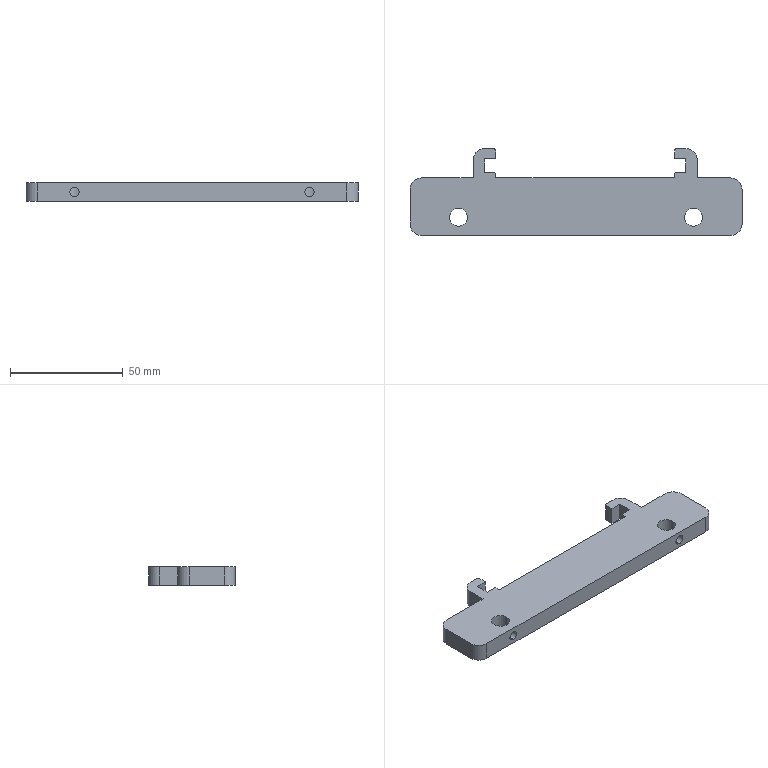Part | SolidWorks | features ICE 5, Fillet 3, Chamfer 1, Extrusion 1, HoleWzd 1, MirrorPattern 1 | 1 solid | 40 faces | box 147 x 38.4 x 8 mm | volume 30280 mm3 | plane 24 | cylinder 16 | commonest cylinder face diameters 10 x6 4.2 x4 8 x4 2 x2
STEP:
#1=CARTESIAN_POINT('',(21.5,-21.4,6.1));
#2=VERTEX_POINT('',#1);
#3=CARTESIAN_POINT('',(21.5,-21.4,1.9));
#4=VERTEX_POINT('',#3);
#5=CARTESIAN_POINT('',(21.5,-21.4,6.1));
#6=CARTESIAN_POINT('',(21.36,-21.4,6.1));
#7=CARTESIAN_POINT('',(21.219,-21.392,6.086));
#8=CARTESIAN_POINT('',(20.946,-21.364,6.03));
#9=CARTESIAN_POINT('',(20.814,-21.343,5.989));
#10=CARTESIAN_POINT('',(20.558,-21.29,5.882));
#11=CARTESIAN_POINT('',(20.438,-21.258,5.817));
#12=CARTESIAN_POINT('',(20.213,-21.189,5.665));
#13=CARTESIAN_POINT('',(20.108,-21.151,5.578));
#14=CARTESIAN_POINT('',(19.918,-21.075,5.387));
#15=CARTESIAN_POINT('',(19.833,-21.037,5.284));
#16=CARTESIAN_POINT('',(19.681,-20.964,5.058));
#17=CARTESIAN_POINT('',(19.616,-20.929,4.938));
#18=CARTESIAN_POINT('',(19.458,-20.842,4.562));
#19=CARTESIAN_POINT('',(19.4,-20.805,4.281));
#20=CARTESIAN_POINT('',(19.4,-20.804,3.864));
#21=CARTESIAN_POINT('',(19.414,-20.813,3.722));
#22=CARTESIAN_POINT('',(19.469,-20.846,3.449));
#23=CARTESIAN_POINT('',(19.509,-20.87,3.317));
#24=CARTESIAN_POINT('',(19.616,-20.929,3.063));
#25=CARTESIAN_POINT('',(19.681,-20.963,2.942));
#26=CARTESIAN_POINT('',(19.831,-21.036,2.718));
#27=CARTESIAN_POINT('',(19.918,-21.075,2.612));
#28=CARTESIAN_POINT('',(20.109,-21.152,2.421));
#29=CARTESIAN_POINT('',(20.212,-21.189,2.336));
#30=CARTESIAN_POINT('',(20.437,-21.258,2.184));
#31=CARTESIAN_POINT('',(20.559,-21.29,2.118));
#32=CARTESIAN_POINT('',(20.811,-21.342,2.011));
#33=CARTESIAN_POINT('',(20.943,-21.363,1.97));
#34=CARTESIAN_POINT('',(21.217,-21.392,1.914));
#35=CARTESIAN_POINT('',(21.359,-21.4,1.9));
#36=CARTESIAN_POINT('',(21.5,-21.4,1.9));
#37=B_SPLINE_CURVE_WITH_KNOTS('',3,(#5,#6,#7,#8,#9,#10,#11,#12,#13,#14,#15,#16,#17,#18,#19,#20,#21,#22,#23,#24,#25,#26,#27,#28,#29,#30,#31,#32,#33,#34,#35,#36),.UNSPECIFIED.,.F.,.F.,(4,2,2,2,2,2,2,2,2,2,2,2,2,2,2,4),(0.006693,0.007111,0.007528,0.007946,0.008363,0.008781,0.009198,0.01003,0.01045,0.01087,0.01129,0.0117,0.01212,0.01254,0.01296,0.01337),.UNSPECIFIED.);
#38=EDGE_CURVE('',#2,#4,#37,.T.);
#39=ORIENTED_EDGE('',*,*,#38,.F.);
#40=CARTESIAN_POINT('',(21.5,-25.4,6.1));
#41=VERTEX_POINT('',#40);
#42=CARTESIAN_POINT('',(21.5,-25.4,6.1));
#43=DIRECTION('',(0.,-1.,0.));
#44=VECTOR('',#43,1000.);
#45=LINE('',#42,#44);
#46=EDGE_CURVE('',#2,#41,#45,.T.);
#47=ORIENTED_EDGE('',*,*,#46,.T.);
#48=CARTESIAN_POINT('',(21.5,-25.4,1.9));
#49=VERTEX_POINT('',#48);
#50=CARTESIAN_POINT('',(21.5,-25.4,4.));
#51=DIRECTION('',(0.,-1.,0.));
#52=DIRECTION('',(0.,0.,-1.));
#53=AXIS2_PLACEMENT_3D('',#50,#51,#52);
#54=CIRCLE('',#53,2.1);
#55=EDGE_CURVE('',#41,#49,#54,.T.);
#56=ORIENTED_EDGE('',*,*,#55,.T.);
#57=CARTESIAN_POINT('',(21.5,-25.4,1.9));
#58=DIRECTION('',(0.,-1.,0.));
#59=VECTOR('',#58,1000.);
#60=LINE('',#57,#59);
#61=EDGE_CURVE('',#4,#49,#60,.T.);
#62=ORIENTED_EDGE('',*,*,#61,.F.);
#63=EDGE_LOOP('',(#39,#47,#56,#62));
#64=FACE_OUTER_BOUND('',#63,.T.);
#65=CARTESIAN_POINT('',(21.5,-25.4,4.));
#66=DIRECTION('',(0.,-1.,0.));
#67=DIRECTION('',(0.,0.,-1.));
#68=AXIS2_PLACEMENT_3D('',#65,#66,#67);
#69=CYLINDRICAL_SURFACE('',#68,2.1);
#70=ADVANCED_FACE('',(#64),#69,.F.);
#71=CARTESIAN_POINT('',(125.5,-21.4,6.1));
#72=VERTEX_POINT('',#71);
#73=CARTESIAN_POINT('',(125.5,-21.4,1.9));
#74=VERTEX_POINT('',#73);
#75=CARTESIAN_POINT('',(125.5,-21.4,6.1));
#76=CARTESIAN_POINT('',(125.36,-21.4,6.1));
#77=CARTESIAN_POINT('',(125.219,-21.392,6.086));
#78=CARTESIAN_POINT('',(124.946,-21.364,6.03));
#79=CARTESIAN_POINT('',(124.814,-21.343,5.989));
#80=CARTESIAN_POINT('',(124.558,-21.29,5.882));
#81=CARTESIAN_POINT('',(124.438,-21.258,5.817));
#82=CARTESIAN_POINT('',(124.213,-21.189,5.665));
#83=CARTESIAN_POINT('',(124.108,-21.151,5.578));
#84=CARTESIAN_POINT('',(123.918,-21.075,5.387));
#85=CARTESIAN_POINT('',(123.833,-21.037,5.284));
#86=CARTESIAN_POINT('',(123.681,-20.964,5.058));
#87=CARTESIAN_POINT('',(123.616,-20.929,4.938));
#88=CARTESIAN_POINT('',(123.458,-20.842,4.562));
#89=CARTESIAN_POINT('',(123.4,-20.805,4.281));
#90=CARTESIAN_POINT('',(123.4,-20.804,3.864));
#91=CARTESIAN_POINT('',(123.414,-20.813,3.722));
#92=CARTESIAN_POINT('',(123.469,-20.846,3.449));
#93=CARTESIAN_POINT('',(123.509,-20.87,3.317));
#94=CARTESIAN_POINT('',(123.616,-20.929,3.063));
#95=CARTESIAN_POINT('',(123.681,-20.963,2.942));
#96=CARTESIAN_POINT('',(123.831,-21.036,2.718));
#97=CARTESIAN_POINT('',(123.918,-21.075,2.612));
#98=CARTESIAN_POINT('',(124.109,-21.152,2.421));
#99=CARTESIAN_POINT('',(124.212,-21.189,2.336));
#100=CARTESIAN_POINT('',(124.437,-21.258,2.184));
#101=CARTESIAN_POINT('',(124.559,-21.29,2.118));
#102=CARTESIAN_POINT('',(124.811,-21.342,2.011));
#103=CARTESIAN_POINT('',(124.943,-21.363,1.97));
#104=CARTESIAN_POINT('',(125.217,-21.392,1.914));
#105=CARTESIAN_POINT('',(125.359,-21.4,1.9));
#106=CARTESIAN_POINT('',(125.5,-21.4,1.9));
#107=B_SPLINE_CURVE_WITH_KNOTS('',3,(#75,#76,#77,#78,#79,#80,#81,#82,#83,#84,#85,#86,#87,#88,#89,#90,#91,#92,#93,#94,#95,#96,#97,#98,#99,#100,#101,#102,#103,#104,#105,#106),.UNSPECIFIED.,.F.,.F.,(4,2,2,2,2,2,2,2,2,2,2,2,2,2,2,4),(0.006693,0.007111,0.007528,0.007946,0.008363,0.008781,0.009198,0.01003,0.01045,0.01087,0.01129,0.0117,0.01212,0.01254,0.01296,0.01337),.UNSPECIFIED.);
#108=EDGE_CURVE('',#72,#74,#107,.T.);
#109=ORIENTED_EDGE('',*,*,#108,.F.);
#110=CARTESIAN_POINT('',(125.5,-25.4,6.1));
#111=VERTEX_POINT('',#110);
#112=CARTESIAN_POINT('',(125.5,-25.4,6.1));
#113=DIRECTION('',(0.,-1.,0.));
#114=VECTOR('',#113,1000.);
#115=LINE('',#112,#114);
#116=EDGE_CURVE('',#72,#111,#115,.T.);
#117=ORIENTED_EDGE('',*,*,#116,.T.);
#118=CARTESIAN_POINT('',(125.5,-25.4,1.9));
#119=VERTEX_POINT('',#118);
#120=CARTESIAN_POINT('',(125.5,-25.4,4.));
#121=DIRECTION('',(0.,-1.,0.));
#122=DIRECTION('',(0.,0.,-1.));
#123=AXIS2_PLACEMENT_3D('',#120,#121,#122);
#124=CIRCLE('',#123,2.1);
#125=EDGE_CURVE('',#111,#119,#124,.T.);
#126=ORIENTED_EDGE('',*,*,#125,.T.);
#127=CARTESIAN_POINT('',(125.5,-25.4,1.9));
#128=DIRECTION('',(0.,-1.,0.));
#129=VECTOR('',#128,1000.);
#130=LINE('',#127,#129);
#131=EDGE_CURVE('',#74,#119,#130,.T.);
#132=ORIENTED_EDGE('',*,*,#131,.F.);
#133=EDGE_LOOP('',(#109,#117,#126,#132));
#134=FACE_OUTER_BOUND('',#133,.T.);
#135=CARTESIAN_POINT('',(125.5,-25.4,4.));
#136=DIRECTION('',(0.,-1.,0.));
#137=DIRECTION('',(0.,0.,-1.));
#138=AXIS2_PLACEMENT_3D('',#135,#136,#137);
#139=CYLINDRICAL_SURFACE('',#138,2.1);
#140=ADVANCED_FACE('',(#134),#139,.F.);
#141=CARTESIAN_POINT('',(21.5,-21.4,1.9));
#142=CARTESIAN_POINT('',(21.642,-21.4,1.9));
#143=CARTESIAN_POINT('',(21.78,-21.393,1.914));
#144=CARTESIAN_POINT('',(22.053,-21.364,1.969));
#145=CARTESIAN_POINT('',(22.187,-21.343,2.011));
#146=CARTESIAN_POINT('',(22.568,-21.264,2.171));
#147=CARTESIAN_POINT('',(22.797,-21.189,2.327));
#148=CARTESIAN_POINT('',(23.082,-21.075,2.612));
#149=CARTESIAN_POINT('',(23.168,-21.036,2.717));
#150=CARTESIAN_POINT('',(23.319,-20.963,2.943));
#151=CARTESIAN_POINT('',(23.384,-20.929,3.062));
#152=CARTESIAN_POINT('',(23.489,-20.871,3.313));
#153=CARTESIAN_POINT('',(23.531,-20.846,3.447));
#154=CARTESIAN_POINT('',(23.586,-20.813,3.72));
#155=CARTESIAN_POINT('',(23.6,-20.805,3.858));
#156=CARTESIAN_POINT('',(23.6,-20.804,4.138));
#157=CARTESIAN_POINT('',(23.586,-20.813,4.28));
#158=CARTESIAN_POINT('',(23.531,-20.846,4.552));
#159=CARTESIAN_POINT('',(23.49,-20.871,4.685));
#160=CARTESIAN_POINT('',(23.383,-20.929,4.939));
#161=CARTESIAN_POINT('',(23.319,-20.964,5.059));
#162=CARTESIAN_POINT('',(23.167,-21.037,5.284));
#163=CARTESIAN_POINT('',(23.08,-21.076,5.389));
#164=CARTESIAN_POINT('',(22.795,-21.19,5.675));
#165=CARTESIAN_POINT('',(22.565,-21.264,5.83));
#166=CARTESIAN_POINT('',(22.187,-21.343,5.989));
#167=CARTESIAN_POINT('',(22.053,-21.364,6.031));
#168=CARTESIAN_POINT('',(21.778,-21.393,6.086));
#169=CARTESIAN_POINT('',(21.64,-21.4,6.1));
#170=CARTESIAN_POINT('',(21.5,-21.4,6.1));
#171=B_SPLINE_CURVE_WITH_KNOTS('',3,(#141,#142,#143,#144,#145,#146,#147,#148,#149,#150,#151,#152,#153,#154,#155,#156,#157,#158,#159,#160,#161,#162,#163,#164,#165,#166,#167,#168,#169,#170),.UNSPECIFIED.,.F.,.F.,(4,2,2,2,2,2,2,2,2,2,2,2,2,2,4),(0.,0.0004183,0.0008367,0.001673,0.002092,0.00251,0.002928,0.003347,0.003765,0.004183,0.004602,0.00502,0.005857,0.006275,0.006693),.UNSPECIFIED.);
#172=EDGE_CURVE('',#4,#2,#171,.T.);
#173=ORIENTED_EDGE('',*,*,#172,.T.);
#174=ORIENTED_EDGE('',*,*,#38,.T.);
#175=EDGE_LOOP('',(#173,#174));
#176=FACE_BOUND('',#175,.T.);
#177=CARTESIAN_POINT('',(17.5,-17.4,0.));
#178=VERTEX_POINT('',#177);
#179=CARTESIAN_POINT('',(25.5,-17.4,0.));
#180=VERTEX_POINT('',#179);
#181=CARTESIAN_POINT('',(21.5,-17.4,0.));
#182=DIRECTION('',(0.,0.,1.));
#183=DIRECTION('',(1.,0.,0.));
#184=AXIS2_PLACEMENT_3D('',#181,#182,#183);
#185=CIRCLE('',#184,4.);
#186=EDGE_CURVE('',#178,#180,#185,.T.);
#187=ORIENTED_EDGE('',*,*,#186,.F.);
#188=CARTESIAN_POINT('',(17.5,-17.4,8.));
#189=VERTEX_POINT('',#188);
#190=CARTESIAN_POINT('',(17.5,-17.4,0.));
#191=DIRECTION('',(0.,0.,1.));
#192=VECTOR('',#191,1000.);
#193=LINE('',#190,#192);
#194=EDGE_CURVE('',#178,#189,#193,.T.);
#195=ORIENTED_EDGE('',*,*,#194,.T.);
#196=CARTESIAN_POINT('',(25.5,-17.4,8.));
#197=VERTEX_POINT('',#196);
#198=CARTESIAN_POINT('',(21.5,-17.4,8.));
#199=DIRECTION('',(0.,0.,1.));
#200=DIRECTION('',(1.,0.,0.));
#201=AXIS2_PLACEMENT_3D('',#198,#199,#200);
#202=CIRCLE('',#201,4.);
#203=EDGE_CURVE('',#189,#197,#202,.T.);
#204=ORIENTED_EDGE('',*,*,#203,.T.);
#205=CARTESIAN_POINT('',(25.5,-17.4,0.));
#206=DIRECTION('',(0.,0.,1.));
#207=VECTOR('',#206,1000.);
#208=LINE('',#205,#207);
#209=EDGE_CURVE('',#180,#197,#208,.T.);
#210=ORIENTED_EDGE('',*,*,#209,.F.);
#211=EDGE_LOOP('',(#187,#195,#204,#210));
#212=FACE_OUTER_BOUND('',#211,.T.);
#213=CARTESIAN_POINT('',(21.5,-17.4,0.));
#214=DIRECTION('',(0.,0.,1.));
#215=DIRECTION('',(1.,0.,0.));
#216=AXIS2_PLACEMENT_3D('',#213,#214,#215);
#217=CYLINDRICAL_SURFACE('',#216,4.);
#218=ADVANCED_FACE('',(#176,#212),#217,.F.);
#219=CARTESIAN_POINT('',(125.5,-21.4,1.9));
#220=CARTESIAN_POINT('',(125.642,-21.4,1.9));
#221=CARTESIAN_POINT('',(125.78,-21.393,1.914));
#222=CARTESIAN_POINT('',(126.053,-21.364,1.969));
#223=CARTESIAN_POINT('',(126.187,-21.343,2.011));
#224=CARTESIAN_POINT('',(126.568,-21.264,2.171));
#225=CARTESIAN_POINT('',(126.797,-21.189,2.327));
#226=CARTESIAN_POINT('',(127.082,-21.075,2.612));
#227=CARTESIAN_POINT('',(127.168,-21.036,2.717));
#228=CARTESIAN_POINT('',(127.319,-20.963,2.943));
#229=CARTESIAN_POINT('',(127.384,-20.929,3.062));
#230=CARTESIAN_POINT('',(127.489,-20.871,3.313));
#231=CARTESIAN_POINT('',(127.531,-20.846,3.447));
#232=CARTESIAN_POINT('',(127.586,-20.813,3.72));
#233=CARTESIAN_POINT('',(127.6,-20.805,3.858));
#234=CARTESIAN_POINT('',(127.6,-20.804,4.138));
#235=CARTESIAN_POINT('',(127.586,-20.813,4.28));
#236=CARTESIAN_POINT('',(127.531,-20.846,4.552));
#237=CARTESIAN_POINT('',(127.49,-20.871,4.685));
#238=CARTESIAN_POINT('',(127.383,-20.929,4.939));
#239=CARTESIAN_POINT('',(127.319,-20.964,5.059));
#240=CARTESIAN_POINT('',(127.167,-21.037,5.284));
#241=CARTESIAN_POINT('',(127.08,-21.076,5.389));
#242=CARTESIAN_POINT('',(126.795,-21.19,5.675));
#243=CARTESIAN_POINT('',(126.565,-21.264,5.83));
#244=CARTESIAN_POINT('',(126.187,-21.343,5.989));
#245=CARTESIAN_POINT('',(126.053,-21.364,6.031));
#246=CARTESIAN_POINT('',(125.778,-21.393,6.086));
#247=CARTESIAN_POINT('',(125.64,-21.4,6.1));
#248=CARTESIAN_POINT('',(125.5,-21.4,6.1));
#249=B_SPLINE_CURVE_WITH_KNOTS('',3,(#219,#220,#221,#222,#223,#224,#225,#226,#227,#228,#229,#230,#231,#232,#233,#234,#235,#236,#237,#238,#239,#240,#241,#242,#243,#244,#245,#246,#247,#248),.UNSPECIFIED.,.F.,.F.,(4,2,2,2,2,2,2,2,2,2,2,2,2,2,4),(0.,0.0004183,0.0008367,0.001673,0.002092,0.00251,0.002928,0.003347,0.003765,0.004183,0.004602,0.00502,0.005857,0.006275,0.006693),.UNSPECIFIED.);
#250=EDGE_CURVE('',#74,#72,#249,.T.);
#251=ORIENTED_EDGE('',*,*,#250,.T.);
#252=ORIENTED_EDGE('',*,*,#108,.T.);
#253=EDGE_LOOP('',(#251,#252));
#254=FACE_BOUND('',#253,.T.);
#255=CARTESIAN_POINT('',(121.5,-17.4,0.));
#256=VERTEX_POINT('',#255);
#257=CARTESIAN_POINT('',(129.5,-17.4,0.));
#258=VERTEX_POINT('',#257);
#259=CARTESIAN_POINT('',(125.5,-17.4,0.));
#260=DIRECTION('',(0.,0.,1.));
#261=DIRECTION('',(1.,0.,0.));
#262=AXIS2_PLACEMENT_3D('',#259,#260,#261);
#263=CIRCLE('',#262,4.);
#264=EDGE_CURVE('',#256,#258,#263,.T.);
#265=ORIENTED_EDGE('',*,*,#264,.F.);
#266=CARTESIAN_POINT('',(121.5,-17.4,8.));
#267=VERTEX_POINT('',#266);
#268=CARTESIAN_POINT('',(121.5,-17.4,0.));
#269=DIRECTION('',(0.,0.,1.));
#270=VECTOR('',#269,1000.);
#271=LINE('',#268,#270);
#272=EDGE_CURVE('',#256,#267,#271,.T.);
#273=ORIENTED_EDGE('',*,*,#272,.T.);
#274=CARTESIAN_POINT('',(129.5,-17.4,8.));
#275=VERTEX_POINT('',#274);
#276=CARTESIAN_POINT('',(125.5,-17.4,8.));
#277=DIRECTION('',(0.,0.,1.));
#278=DIRECTION('',(1.,0.,0.));
#279=AXIS2_PLACEMENT_3D('',#276,#277,#278);
#280=CIRCLE('',#279,4.);
#281=EDGE_CURVE('',#267,#275,#280,.T.);
#282=ORIENTED_EDGE('',*,*,#281,.T.);
#283=CARTESIAN_POINT('',(129.5,-17.4,0.));
#284=DIRECTION('',(0.,0.,1.));
#285=VECTOR('',#284,1000.);
#286=LINE('',#283,#285);
#287=EDGE_CURVE('',#258,#275,#286,.T.);
#288=ORIENTED_EDGE('',*,*,#287,.F.);
#289=EDGE_LOOP('',(#265,#273,#282,#288));
#290=FACE_OUTER_BOUND('',#289,.T.);
#291=CARTESIAN_POINT('',(125.5,-17.4,0.));
#292=DIRECTION('',(0.,0.,1.));
#293=DIRECTION('',(1.,0.,0.));
#294=AXIS2_PLACEMENT_3D('',#291,#292,#293);
#295=CYLINDRICAL_SURFACE('',#294,4.);
#296=ADVANCED_FACE('',(#254,#290),#295,.F.);
#297=CARTESIAN_POINT('',(117.2,0.,0.));
#298=VERTEX_POINT('',#297);
#299=CARTESIAN_POINT('',(117.2,0.,8.));
#300=VERTEX_POINT('',#299);
#301=CARTESIAN_POINT('',(117.2,0.,0.));
#302=DIRECTION('',(0.,0.,1.));
#303=VECTOR('',#302,1000.);
#304=LINE('',#301,#303);
#305=EDGE_CURVE('',#298,#300,#304,.T.);
#306=ORIENTED_EDGE('',*,*,#305,.F.);
#307=CARTESIAN_POINT('',(38.,0.,0.));
#308=VERTEX_POINT('',#307);
#309=CARTESIAN_POINT('',(0.,0.,0.));
#310=DIRECTION('',(-1.,0.,0.));
#311=VECTOR('',#310,1000.);
#312=LINE('',#309,#311);
#313=EDGE_CURVE('',#298,#308,#312,.T.);
#314=ORIENTED_EDGE('',*,*,#313,.T.);
#315=CARTESIAN_POINT('',(38.,0.,8.));
#316=VERTEX_POINT('',#315);
#317=CARTESIAN_POINT('',(38.,0.,0.));
#318=DIRECTION('',(0.,0.,-1.));
#319=VECTOR('',#318,1000.);
#320=LINE('',#317,#319);
#321=EDGE_CURVE('',#316,#308,#320,.T.);
#322=ORIENTED_EDGE('',*,*,#321,.F.);
#323=CARTESIAN_POINT('',(0.,0.,8.));
#324=DIRECTION('',(-1.,0.,0.));
#325=VECTOR('',#324,1000.);
#326=LINE('',#323,#325);
#327=EDGE_CURVE('',#300,#316,#326,.T.);
#328=ORIENTED_EDGE('',*,*,#327,.F.);
#329=EDGE_LOOP('',(#306,#314,#322,#328));
#330=FACE_OUTER_BOUND('',#329,.T.);
#331=CARTESIAN_POINT('',(0.,0.,8.));
#332=DIRECTION('',(0.,-1.,0.));
#333=DIRECTION('',(0.,0.,-1.));
#334=AXIS2_PLACEMENT_3D('',#331,#332,#333);
#335=PLANE('',#334);
#336=ADVANCED_FACE('',(#330),#335,.F.);
#337=CARTESIAN_POINT('',(33.,8.5,8.));
#338=VERTEX_POINT('',#337);
#339=CARTESIAN_POINT('',(33.,2.4,8.));
#340=VERTEX_POINT('',#339);
#341=CARTESIAN_POINT('',(33.,10.,8.));
#342=DIRECTION('',(0.,-1.,0.));
#343=VECTOR('',#342,1000.);
#344=LINE('',#341,#343);
#345=EDGE_CURVE('',#338,#340,#344,.T.);
#346=ORIENTED_EDGE('',*,*,#345,.T.);
#347=CARTESIAN_POINT('',(33.,2.4,0.));
#348=VERTEX_POINT('',#347);
#349=CARTESIAN_POINT('',(33.,2.4,0.));
#350=DIRECTION('',(0.,0.,1.));
#351=VECTOR('',#350,1000.);
#352=LINE('',#349,#351);
#353=EDGE_CURVE('',#348,#340,#352,.T.);
#354=ORIENTED_EDGE('',*,*,#353,.F.);
#355=CARTESIAN_POINT('',(33.,8.5,0.));
#356=VERTEX_POINT('',#355);
#357=CARTESIAN_POINT('',(33.,10.,0.));
#358=DIRECTION('',(0.,-1.,0.));
#359=VECTOR('',#358,1000.);
#360=LINE('',#357,#359);
#361=EDGE_CURVE('',#356,#348,#360,.T.);
#362=ORIENTED_EDGE('',*,*,#361,.F.);
#363=CARTESIAN_POINT('',(33.,8.5,8.));
#364=DIRECTION('',(0.,0.,-1.));
#365=VECTOR('',#364,1000.);
#366=LINE('',#363,#365);
#367=EDGE_CURVE('',#338,#356,#366,.T.);
#368=ORIENTED_EDGE('',*,*,#367,.F.);
#369=EDGE_LOOP('',(#346,#354,#362,#368));
#370=FACE_OUTER_BOUND('',#369,.T.);
#371=CARTESIAN_POINT('',(33.,10.,0.));
#372=DIRECTION('',(-1.,0.,0.));
#373=DIRECTION('',(0.,0.,1.));
#374=AXIS2_PLACEMENT_3D('',#371,#372,#373);
#375=PLANE('',#374);
#376=ADVANCED_FACE('',(#370),#375,.F.);
#377=CARTESIAN_POINT('',(28.,0.,0.));
#378=VERTEX_POINT('',#377);
#379=CARTESIAN_POINT('',(5.,0.,0.));
#380=VERTEX_POINT('',#379);
#381=CARTESIAN_POINT('',(0.,0.,0.));
#382=DIRECTION('',(-1.,0.,0.));
#383=VECTOR('',#382,1000.);
#384=LINE('',#381,#383);
#385=EDGE_CURVE('',#378,#380,#384,.T.);
#386=ORIENTED_EDGE('',*,*,#385,.T.);
#387=CARTESIAN_POINT('',(5.,0.,8.));
#388=VERTEX_POINT('',#387);
#389=CARTESIAN_POINT('',(5.,0.,8.));
#390=DIRECTION('',(0.,0.,1.));
#391=VECTOR('',#390,1000.);
#392=LINE('',#389,#391);
#393=EDGE_CURVE('',#380,#388,#392,.T.);
#394=ORIENTED_EDGE('',*,*,#393,.T.);
#395=CARTESIAN_POINT('',(28.,0.,8.));
#396=VERTEX_POINT('',#395);
#397=CARTESIAN_POINT('',(0.,0.,8.));
#398=DIRECTION('',(-1.,0.,0.));
#399=VECTOR('',#398,1000.);
#400=LINE('',#397,#399);
#401=EDGE_CURVE('',#396,#388,#400,.T.);
#402=ORIENTED_EDGE('',*,*,#401,.F.);
#403=CARTESIAN_POINT('',(28.,0.,0.));
#404=DIRECTION('',(0.,0.,1.));
#405=VECTOR('',#404,1000.);
#406=LINE('',#403,#405);
#407=EDGE_CURVE('',#378,#396,#406,.T.);
#408=ORIENTED_EDGE('',*,*,#407,.F.);
#409=EDGE_LOOP('',(#386,#394,#402,#408));
#410=FACE_OUTER_BOUND('',#409,.T.);
#411=CARTESIAN_POINT('',(0.,0.,8.));
#412=DIRECTION('',(0.,-1.,0.));
#413=DIRECTION('',(0.,0.,-1.));
#414=AXIS2_PLACEMENT_3D('',#411,#412,#413);
#415=PLANE('',#414);
#416=ADVANCED_FACE('',(#410),#415,.F.);
#417=CARTESIAN_POINT('',(142.,0.,8.));
#418=VERTEX_POINT('',#417);
#419=CARTESIAN_POINT('',(127.2,0.,8.));
#420=VERTEX_POINT('',#419);
#421=CARTESIAN_POINT('',(0.,0.,8.));
#422=DIRECTION('',(-1.,0.,0.));
#423=VECTOR('',#422,1000.);
#424=LINE('',#421,#423);
#425=EDGE_CURVE('',#418,#420,#424,.T.);
#426=ORIENTED_EDGE('',*,*,#425,.F.);
#427=CARTESIAN_POINT('',(142.,0.,0.));
#428=VERTEX_POINT('',#427);
#429=CARTESIAN_POINT('',(142.,0.,8.));
#430=DIRECTION('',(0.,0.,-1.));
#431=VECTOR('',#430,1000.);
#432=LINE('',#429,#431);
#433=EDGE_CURVE('',#418,#428,#432,.T.);
#434=ORIENTED_EDGE('',*,*,#433,.T.);
#435=CARTESIAN_POINT('',(127.2,0.,0.));
#436=VERTEX_POINT('',#435);
#437=CARTESIAN_POINT('',(0.,0.,0.));
#438=DIRECTION('',(-1.,0.,0.));
#439=VECTOR('',#438,1000.);
#440=LINE('',#437,#439);
#441=EDGE_CURVE('',#428,#436,#440,.T.);
#442=ORIENTED_EDGE('',*,*,#441,.T.);
#443=CARTESIAN_POINT('',(127.2,0.,0.));
#444=DIRECTION('',(0.,0.,-1.));
#445=VECTOR('',#444,1000.);
#446=LINE('',#443,#445);
#447=EDGE_CURVE('',#420,#436,#446,.T.);
#448=ORIENTED_EDGE('',*,*,#447,.F.);
#449=EDGE_LOOP('',(#426,#434,#442,#448));
#450=FACE_OUTER_BOUND('',#449,.T.);
#451=CARTESIAN_POINT('',(0.,0.,8.));
#452=DIRECTION('',(0.,-1.,0.));
#453=DIRECTION('',(0.,0.,-1.));
#454=AXIS2_PLACEMENT_3D('',#451,#452,#453);
#455=PLANE('',#454);
#456=ADVANCED_FACE('',(#450),#455,.F.);
#457=CARTESIAN_POINT('',(0.,-5.,0.));
#458=VERTEX_POINT('',#457);
#459=CARTESIAN_POINT('',(0.,-20.4,0.));
#460=VERTEX_POINT('',#459);
#461=CARTESIAN_POINT('',(0.,0.,0.));
#462=DIRECTION('',(0.,-1.,0.));
#463=VECTOR('',#462,1000.);
#464=LINE('',#461,#463);
#465=EDGE_CURVE('',#458,#460,#464,.T.);
#466=ORIENTED_EDGE('',*,*,#465,.T.);
#467=CARTESIAN_POINT('',(0.,-20.4,8.));
#468=VERTEX_POINT('',#467);
#469=CARTESIAN_POINT('',(0.,-20.4,8.));
#470=DIRECTION('',(0.,0.,1.));
#471=VECTOR('',#470,1000.);
#472=LINE('',#469,#471);
#473=EDGE_CURVE('',#460,#468,#472,.T.);
#474=ORIENTED_EDGE('',*,*,#473,.T.);
#475=CARTESIAN_POINT('',(0.,-5.,8.));
#476=VERTEX_POINT('',#475);
#477=CARTESIAN_POINT('',(0.,0.,8.));
#478=DIRECTION('',(0.,-1.,0.));
#479=VECTOR('',#478,1000.);
#480=LINE('',#477,#479);
#481=EDGE_CURVE('',#476,#468,#480,.T.);
#482=ORIENTED_EDGE('',*,*,#481,.F.);
#483=CARTESIAN_POINT('',(0.,-5.,8.));
#484=DIRECTION('',(0.,0.,-1.));
#485=VECTOR('',#484,1000.);
#486=LINE('',#483,#485);
#487=EDGE_CURVE('',#476,#458,#486,.T.);
#488=ORIENTED_EDGE('',*,*,#487,.T.);
#489=EDGE_LOOP('',(#466,#474,#482,#488));
#490=FACE_OUTER_BOUND('',#489,.T.);
#491=CARTESIAN_POINT('',(0.,0.,8.));
#492=DIRECTION('',(1.,0.,0.));
#493=DIRECTION('',(0.,1.,0.));
#494=AXIS2_PLACEMENT_3D('',#491,#492,#493);
#495=PLANE('',#494);
#496=ADVANCED_FACE('',(#490),#495,.F.);
#497=CARTESIAN_POINT('',(21.5,-25.4,4.));
#498=DIRECTION('',(0.,-1.,0.));
#499=DIRECTION('',(0.,0.,-1.));
#500=AXIS2_PLACEMENT_3D('',#497,#498,#499);
#501=CIRCLE('',#500,2.1);
#502=EDGE_CURVE('',#49,#41,#501,.T.);
#503=ORIENTED_EDGE('',*,*,#502,.F.);
#504=ORIENTED_EDGE('',*,*,#55,.F.);
#505=EDGE_LOOP('',(#503,#504));
#506=FACE_BOUND('',#505,.T.);
#507=CARTESIAN_POINT('',(125.5,-25.4,4.));
#508=DIRECTION('',(0.,-1.,0.));
#509=DIRECTION('',(0.,0.,-1.));
#510=AXIS2_PLACEMENT_3D('',#507,#508,#509);
#511=CIRCLE('',#510,2.1);
#512=EDGE_CURVE('',#119,#111,#511,.T.);
#513=ORIENTED_EDGE('',*,*,#512,.F.);
#514=ORIENTED_EDGE('',*,*,#125,.F.);
#515=EDGE_LOOP('',(#513,#514));
#516=FACE_BOUND('',#515,.T.);
#517=CARTESIAN_POINT('',(5.,-25.4,0.));
#518=VERTEX_POINT('',#517);
#519=CARTESIAN_POINT('',(142.,-25.4,0.));
#520=VERTEX_POINT('',#519);
#521=CARTESIAN_POINT('',(0.,-25.4,0.));
#522=DIRECTION('',(1.,0.,0.));
#523=VECTOR('',#522,1000.);
#524=LINE('',#521,#523);
#525=EDGE_CURVE('',#518,#520,#524,.T.);
#526=ORIENTED_EDGE('',*,*,#525,.T.);
#527=CARTESIAN_POINT('',(142.,-25.4,8.));
#528=VERTEX_POINT('',#527);
#529=CARTESIAN_POINT('',(142.,-25.4,8.));
#530=DIRECTION('',(0.,0.,1.));
#531=VECTOR('',#530,1000.);
#532=LINE('',#529,#531);
#533=EDGE_CURVE('',#520,#528,#532,.T.);
#534=ORIENTED_EDGE('',*,*,#533,.T.);
#535=CARTESIAN_POINT('',(5.,-25.4,8.));
#536=VERTEX_POINT('',#535);
#537=CARTESIAN_POINT('',(0.,-25.4,8.));
#538=DIRECTION('',(1.,0.,0.));
#539=VECTOR('',#538,1000.);
#540=LINE('',#537,#539);
#541=EDGE_CURVE('',#536,#528,#540,.T.);
#542=ORIENTED_EDGE('',*,*,#541,.F.);
#543=CARTESIAN_POINT('',(5.,-25.4,8.));
#544=DIRECTION('',(0.,0.,-1.));
#545=VECTOR('',#544,1000.);
#546=LINE('',#543,#545);
#547=EDGE_CURVE('',#536,#518,#546,.T.);
#548=ORIENTED_EDGE('',*,*,#547,.T.);
#549=EDGE_LOOP('',(#526,#534,#542,#548));
#550=FACE_OUTER_BOUND('',#549,.T.);
#551=CARTESIAN_POINT('',(0.,-25.4,8.));
#552=DIRECTION('',(0.,1.,0.));
#553=DIRECTION('',(0.,0.,1.));
#554=AXIS2_PLACEMENT_3D('',#551,#552,#553);
#555=PLANE('',#554);
#556=ADVANCED_FACE('',(#506,#516,#550),#555,.F.);
#557=CARTESIAN_POINT('',(147.,-20.4,8.));
#558=VERTEX_POINT('',#557);
#559=CARTESIAN_POINT('',(147.,-5.,8.));
#560=VERTEX_POINT('',#559);
#561=CARTESIAN_POINT('',(147.,0.,8.));
#562=DIRECTION('',(0.,1.,0.));
#563=VECTOR('',#562,1000.);
#564=LINE('',#561,#563);
#565=EDGE_CURVE('',#558,#560,#564,.T.);
#566=ORIENTED_EDGE('',*,*,#565,.F.);
#567=CARTESIAN_POINT('',(147.,-20.4,0.));
#568=VERTEX_POINT('',#567);
#569=CARTESIAN_POINT('',(147.,-20.4,8.));
#570=DIRECTION('',(0.,0.,-1.));
#571=VECTOR('',#570,1000.);
#572=LINE('',#569,#571);
#573=EDGE_CURVE('',#558,#568,#572,.T.);
#574=ORIENTED_EDGE('',*,*,#573,.T.);
#575=CARTESIAN_POINT('',(147.,-5.,0.));
#576=VERTEX_POINT('',#575);
#577=CARTESIAN_POINT('',(147.,0.,0.));
#578=DIRECTION('',(0.,1.,0.));
#579=VECTOR('',#578,1000.);
#580=LINE('',#577,#579);
#581=EDGE_CURVE('',#568,#576,#580,.T.);
#582=ORIENTED_EDGE('',*,*,#581,.T.);
#583=CARTESIAN_POINT('',(147.,-5.,8.));
#584=DIRECTION('',(0.,0.,1.));
#585=VECTOR('',#584,1000.);
#586=LINE('',#583,#585);
#587=EDGE_CURVE('',#576,#560,#586,.T.);
#588=ORIENTED_EDGE('',*,*,#587,.T.);
#589=EDGE_LOOP('',(#566,#574,#582,#588));
#590=FACE_OUTER_BOUND('',#589,.T.);
#591=CARTESIAN_POINT('',(147.,0.,8.));
#592=DIRECTION('',(-1.,0.,0.));
#593=DIRECTION('',(0.,0.,1.));
#594=AXIS2_PLACEMENT_3D('',#591,#592,#593);
#595=PLANE('',#594);
#596=ADVANCED_FACE('',(#590),#595,.F.);
#597=CARTESIAN_POINT('',(21.5,-17.4,8.));
#598=DIRECTION('',(0.,0.,1.));
#599=DIRECTION('',(1.,0.,0.));
#600=AXIS2_PLACEMENT_3D('',#597,#598,#599);
#601=CIRCLE('',#600,4.);
#602=EDGE_CURVE('',#197,#189,#601,.T.);
#603=ORIENTED_EDGE('',*,*,#602,.F.);
#604=ORIENTED_EDGE('',*,*,#203,.F.);
#605=EDGE_LOOP('',(#603,#604));
#606=FACE_BOUND('',#605,.T.);
#607=CARTESIAN_POINT('',(125.5,-17.4,8.));
#608=DIRECTION('',(0.,0.,1.));
#609=DIRECTION('',(1.,0.,0.));
#610=AXIS2_PLACEMENT_3D('',#607,#608,#609);
#611=CIRCLE('',#610,4.);
#612=EDGE_CURVE('',#275,#267,#611,.T.);
#613=ORIENTED_EDGE('',*,*,#612,.F.);
#614=ORIENTED_EDGE('',*,*,#281,.F.);
#615=EDGE_LOOP('',(#613,#614));
#616=FACE_BOUND('',#615,.T.);
#617=CARTESIAN_POINT('',(118.2,13.,8.));
#618=VERTEX_POINT('',#617);
#619=CARTESIAN_POINT('',(122.2,13.,8.));
#620=VERTEX_POINT('',#619);
#621=CARTESIAN_POINT('',(117.2,13.,8.));
#622=DIRECTION('',(1.,0.,0.));
#623=VECTOR('',#622,1000.);
#624=LINE('',#621,#623);
#625=EDGE_CURVE('',#618,#620,#624,.T.);
#626=ORIENTED_EDGE('',*,*,#625,.F.);
#627=CARTESIAN_POINT('',(117.2,12.,8.));
#628=VERTEX_POINT('',#627);
#629=CARTESIAN_POINT('',(118.2,12.,8.));
#630=DIRECTION('',(0.,0.,1.));
#631=DIRECTION('',(1.,0.,0.));
#632=AXIS2_PLACEMENT_3D('',#629,#630,#631);
#633=CIRCLE('',#632,1.);
#634=EDGE_CURVE('',#618,#628,#633,.T.);
#635=ORIENTED_EDGE('',*,*,#634,.T.);
#636=CARTESIAN_POINT('',(117.2,8.5,8.));
#637=VERTEX_POINT('',#636);
#638=CARTESIAN_POINT('',(117.2,10.,8.));
#639=DIRECTION('',(0.,-1.,0.));
#640=VECTOR('',#639,1000.);
#641=LINE('',#638,#640);
#642=EDGE_CURVE('',#628,#637,#641,.T.);
#643=ORIENTED_EDGE('',*,*,#642,.T.);
#644=CARTESIAN_POINT('',(122.2,8.5,8.));
#645=VERTEX_POINT('',#644);
#646=CARTESIAN_POINT('',(117.2,8.5,8.));
#647=DIRECTION('',(1.,0.,0.));
#648=VECTOR('',#647,1000.);
#649=LINE('',#646,#648);
#650=EDGE_CURVE('',#637,#645,#649,.T.);
#651=ORIENTED_EDGE('',*,*,#650,.T.);
#652=CARTESIAN_POINT('',(122.2,2.4,8.));
#653=VERTEX_POINT('',#652);
#654=CARTESIAN_POINT('',(122.2,10.,8.));
#655=DIRECTION('',(0.,-1.,0.));
#656=VECTOR('',#655,1000.);
#657=LINE('',#654,#656);
#658=EDGE_CURVE('',#645,#653,#657,.T.);
#659=ORIENTED_EDGE('',*,*,#658,.T.);
#660=CARTESIAN_POINT('',(117.7,2.4,8.));
#661=VERTEX_POINT('',#660);
#662=CARTESIAN_POINT('',(117.2,2.4,8.));
#663=DIRECTION('',(1.,0.,0.));
#664=VECTOR('',#663,1000.);
#665=LINE('',#662,#664);
#666=EDGE_CURVE('',#661,#653,#665,.T.);
#667=ORIENTED_EDGE('',*,*,#666,.F.);
#668=CARTESIAN_POINT('',(117.2,1.9,8.));
#669=VERTEX_POINT('',#668);
#670=CARTESIAN_POINT('',(57.65,-57.65,8.));
#671=DIRECTION('',(-0.7071,-0.7071,0.));
#672=VECTOR('',#671,1000.);
#673=LINE('',#670,#672);
#674=EDGE_CURVE('',#661,#669,#673,.T.);
#675=ORIENTED_EDGE('',*,*,#674,.T.);
#676=CARTESIAN_POINT('',(117.2,2.4,8.));
#677=DIRECTION('',(0.,-1.,0.));
#678=VECTOR('',#677,1000.);
#679=LINE('',#676,#678);
#680=EDGE_CURVE('',#669,#300,#679,.T.);
#681=ORIENTED_EDGE('',*,*,#680,.T.);
#682=ORIENTED_EDGE('',*,*,#327,.T.);
#683=CARTESIAN_POINT('',(38.,1.9,8.));
#684=VERTEX_POINT('',#683);
#685=CARTESIAN_POINT('',(38.,2.4,8.));
#686=DIRECTION('',(0.,-1.,0.));
#687=VECTOR('',#686,1000.);
#688=LINE('',#685,#687);
#689=EDGE_CURVE('',#684,#316,#688,.T.);
#690=ORIENTED_EDGE('',*,*,#689,.F.);
#691=CARTESIAN_POINT('',(37.5,2.4,8.));
#692=VERTEX_POINT('',#691);
#693=CARTESIAN_POINT('',(19.95,19.95,8.));
#694=DIRECTION('',(-0.7071,0.7071,0.));
#695=VECTOR('',#694,1000.);
#696=LINE('',#693,#695);
#697=EDGE_CURVE('',#684,#692,#696,.T.);
#698=ORIENTED_EDGE('',*,*,#697,.T.);
#699=CARTESIAN_POINT('',(33.,2.4,8.));
#700=DIRECTION('',(1.,0.,0.));
#701=VECTOR('',#700,1000.);
#702=LINE('',#699,#701);
#703=EDGE_CURVE('',#340,#692,#702,.T.);
#704=ORIENTED_EDGE('',*,*,#703,.F.);
#705=ORIENTED_EDGE('',*,*,#345,.F.);
#706=CARTESIAN_POINT('',(38.,8.5,8.));
#707=VERTEX_POINT('',#706);
#708=CARTESIAN_POINT('',(38.,8.5,8.));
#709=DIRECTION('',(-1.,0.,0.));
#710=VECTOR('',#709,1000.);
#711=LINE('',#708,#710);
#712=EDGE_CURVE('',#707,#338,#711,.T.);
#713=ORIENTED_EDGE('',*,*,#712,.F.);
#714=CARTESIAN_POINT('',(38.,12.,8.));
#715=VERTEX_POINT('',#714);
#716=CARTESIAN_POINT('',(38.,10.,8.));
#717=DIRECTION('',(0.,-1.,0.));
#718=VECTOR('',#717,1000.);
#719=LINE('',#716,#718);
#720=EDGE_CURVE('',#715,#707,#719,.T.);
#721=ORIENTED_EDGE('',*,*,#720,.F.);
#722=CARTESIAN_POINT('',(37.,13.,8.));
#723=VERTEX_POINT('',#722);
#724=CARTESIAN_POINT('',(37.,12.,8.));
#725=DIRECTION('',(0.,0.,1.));
#726=DIRECTION('',(1.,0.,0.));
#727=AXIS2_PLACEMENT_3D('',#724,#725,#726);
#728=CIRCLE('',#727,1.);
#729=EDGE_CURVE('',#715,#723,#728,.T.);
#730=ORIENTED_EDGE('',*,*,#729,.T.);
#731=CARTESIAN_POINT('',(33.,13.,8.));
#732=VERTEX_POINT('',#731);
#733=CARTESIAN_POINT('',(28.,13.,8.));
#734=DIRECTION('',(1.,0.,0.));
#735=VECTOR('',#734,1000.);
#736=LINE('',#733,#735);
#737=EDGE_CURVE('',#732,#723,#736,.T.);
#738=ORIENTED_EDGE('',*,*,#737,.F.);
#739=CARTESIAN_POINT('',(28.,8.,8.));
#740=VERTEX_POINT('',#739);
#741=CARTESIAN_POINT('',(33.,8.,8.));
#742=DIRECTION('',(0.,0.,1.));
#743=DIRECTION('',(1.,0.,0.));
#744=AXIS2_PLACEMENT_3D('',#741,#742,#743);
#745=CIRCLE('',#744,5.);
#746=EDGE_CURVE('',#732,#740,#745,.T.);
#747=ORIENTED_EDGE('',*,*,#746,.T.);
#748=CARTESIAN_POINT('',(28.,10.,8.));
#749=DIRECTION('',(0.,-1.,0.));
#750=VECTOR('',#749,1000.);
#751=LINE('',#748,#750);
#752=EDGE_CURVE('',#740,#396,#751,.T.);
#753=ORIENTED_EDGE('',*,*,#752,.T.);
#754=ORIENTED_EDGE('',*,*,#401,.T.);
#755=CARTESIAN_POINT('',(5.,-5.,8.));
#756=DIRECTION('',(0.,0.,1.));
#757=DIRECTION('',(1.,0.,0.));
#758=AXIS2_PLACEMENT_3D('',#755,#756,#757);
#759=CIRCLE('',#758,5.);
#760=EDGE_CURVE('',#388,#476,#759,.T.);
#761=ORIENTED_EDGE('',*,*,#760,.T.);
#762=ORIENTED_EDGE('',*,*,#481,.T.);
#763=CARTESIAN_POINT('',(5.,-20.4,8.));
#764=DIRECTION('',(0.,0.,1.));
#765=DIRECTION('',(1.,0.,0.));
#766=AXIS2_PLACEMENT_3D('',#763,#764,#765);
#767=CIRCLE('',#766,5.);
#768=EDGE_CURVE('',#468,#536,#767,.T.);
#769=ORIENTED_EDGE('',*,*,#768,.T.);
#770=ORIENTED_EDGE('',*,*,#541,.T.);
#771=CARTESIAN_POINT('',(142.,-20.4,8.));
#772=DIRECTION('',(0.,0.,1.));
#773=DIRECTION('',(1.,0.,0.));
#774=AXIS2_PLACEMENT_3D('',#771,#772,#773);
#775=CIRCLE('',#774,5.);
#776=EDGE_CURVE('',#528,#558,#775,.T.);
#777=ORIENTED_EDGE('',*,*,#776,.T.);
#778=ORIENTED_EDGE('',*,*,#565,.T.);
#779=CARTESIAN_POINT('',(142.,-5.,8.));
#780=DIRECTION('',(0.,0.,1.));
#781=DIRECTION('',(1.,0.,0.));
#782=AXIS2_PLACEMENT_3D('',#779,#780,#781);
#783=CIRCLE('',#782,5.);
#784=EDGE_CURVE('',#560,#418,#783,.T.);
#785=ORIENTED_EDGE('',*,*,#784,.T.);
#786=ORIENTED_EDGE('',*,*,#425,.T.);
#787=CARTESIAN_POINT('',(127.2,8.,8.));
#788=VERTEX_POINT('',#787);
#789=CARTESIAN_POINT('',(127.2,10.,8.));
#790=DIRECTION('',(0.,-1.,0.));
#791=VECTOR('',#790,1000.);
#792=LINE('',#789,#791);
#793=EDGE_CURVE('',#788,#420,#792,.T.);
#794=ORIENTED_EDGE('',*,*,#793,.F.);
#795=CARTESIAN_POINT('',(122.2,8.,8.));
#796=DIRECTION('',(0.,0.,1.));
#797=DIRECTION('',(1.,0.,0.));
#798=AXIS2_PLACEMENT_3D('',#795,#796,#797);
#799=CIRCLE('',#798,5.);
#800=EDGE_CURVE('',#788,#620,#799,.T.);
#801=ORIENTED_EDGE('',*,*,#800,.T.);
#802=EDGE_LOOP('',(#626,#635,#643,#651,#659,#667,#675,#681,#682,#690,#698,#704,#705,#713,#721,#730,#738,#747,#753,#754,#761,#762,#769,#770,#777,#778,#785,#786,#794,#801));
#803=FACE_OUTER_BOUND('',#802,.T.);
#804=CARTESIAN_POINT('',(0.,0.,8.));
#805=DIRECTION('',(0.,0.,1.));
#806=DIRECTION('',(1.,0.,0.));
#807=AXIS2_PLACEMENT_3D('',#804,#805,#806);
#808=PLANE('',#807);
#809=ADVANCED_FACE('',(#606,#616,#803),#808,.T.);
#810=CARTESIAN_POINT('',(21.5,-17.4,0.));
#811=DIRECTION('',(0.,0.,1.));
#812=DIRECTION('',(1.,0.,0.));
#813=AXIS2_PLACEMENT_3D('',#810,#811,#812);
#814=CIRCLE('',#813,4.);
#815=EDGE_CURVE('',#180,#178,#814,.T.);
#816=ORIENTED_EDGE('',*,*,#815,.T.);
#817=ORIENTED_EDGE('',*,*,#186,.T.);
#818=EDGE_LOOP('',(#816,#817));
#819=FACE_BOUND('',#818,.T.);
#820=CARTESIAN_POINT('',(125.5,-17.4,0.));
#821=DIRECTION('',(0.,0.,1.));
#822=DIRECTION('',(1.,0.,0.));
#823=AXIS2_PLACEMENT_3D('',#820,#821,#822);
#824=CIRCLE('',#823,4.);
#825=EDGE_CURVE('',#258,#256,#824,.T.);
#826=ORIENTED_EDGE('',*,*,#825,.T.);
#827=ORIENTED_EDGE('',*,*,#264,.T.);
#828=EDGE_LOOP('',(#826,#827));
#829=FACE_BOUND('',#828,.T.);
#830=CARTESIAN_POINT('',(117.2,8.5,0.));
#831=VERTEX_POINT('',#830);
#832=CARTESIAN_POINT('',(117.2,12.,0.));
#833=VERTEX_POINT('',#832);
#834=CARTESIAN_POINT('',(117.2,10.,0.));
#835=DIRECTION('',(0.,1.,0.));
#836=VECTOR('',#835,1000.);
#837=LINE('',#834,#836);
#838=EDGE_CURVE('',#831,#833,#837,.T.);
#839=ORIENTED_EDGE('',*,*,#838,.T.);
#840=CARTESIAN_POINT('',(118.2,13.,0.));
#841=VERTEX_POINT('',#840);
#842=CARTESIAN_POINT('',(118.2,12.,0.));
#843=DIRECTION('',(0.,0.,-1.));
#844=DIRECTION('',(1.,0.,0.));
#845=AXIS2_PLACEMENT_3D('',#842,#843,#844);
#846=CIRCLE('',#845,1.);
#847=EDGE_CURVE('',#833,#841,#846,.T.);
#848=ORIENTED_EDGE('',*,*,#847,.T.);
#849=CARTESIAN_POINT('',(122.2,13.,0.));
#850=VERTEX_POINT('',#849);
#851=CARTESIAN_POINT('',(127.2,13.,0.));
#852=DIRECTION('',(-1.,0.,0.));
#853=VECTOR('',#852,1000.);
#854=LINE('',#851,#853);
#855=EDGE_CURVE('',#850,#841,#854,.T.);
#856=ORIENTED_EDGE('',*,*,#855,.F.);
#857=CARTESIAN_POINT('',(127.2,8.,0.));
#858=VERTEX_POINT('',#857);
#859=CARTESIAN_POINT('',(122.2,8.,0.));
#860=DIRECTION('',(0.,0.,-1.));
#861=DIRECTION('',(1.,0.,0.));
#862=AXIS2_PLACEMENT_3D('',#859,#860,#861);
#863=CIRCLE('',#862,5.);
#864=EDGE_CURVE('',#850,#858,#863,.T.);
#865=ORIENTED_EDGE('',*,*,#864,.T.);
#866=CARTESIAN_POINT('',(127.2,10.,0.));
#867=DIRECTION('',(0.,-1.,0.));
#868=VECTOR('',#867,1000.);
#869=LINE('',#866,#868);
#870=EDGE_CURVE('',#858,#436,#869,.T.);
#871=ORIENTED_EDGE('',*,*,#870,.T.);
#872=ORIENTED_EDGE('',*,*,#441,.F.);
#873=CARTESIAN_POINT('',(142.,-5.,0.));
#874=DIRECTION('',(0.,0.,-1.));
#875=DIRECTION('',(1.,0.,0.));
#876=AXIS2_PLACEMENT_3D('',#873,#874,#875);
#877=CIRCLE('',#876,5.);
#878=EDGE_CURVE('',#428,#576,#877,.T.);
#879=ORIENTED_EDGE('',*,*,#878,.T.);
#880=ORIENTED_EDGE('',*,*,#581,.F.);
#881=CARTESIAN_POINT('',(142.,-20.4,0.));
#882=DIRECTION('',(0.,0.,-1.));
#883=DIRECTION('',(1.,0.,0.));
#884=AXIS2_PLACEMENT_3D('',#881,#882,#883);
#885=CIRCLE('',#884,5.);
#886=EDGE_CURVE('',#568,#520,#885,.T.);
#887=ORIENTED_EDGE('',*,*,#886,.T.);
#888=ORIENTED_EDGE('',*,*,#525,.F.);
#889=CARTESIAN_POINT('',(5.,-20.4,0.));
#890=DIRECTION('',(0.,0.,-1.));
#891=DIRECTION('',(1.,0.,0.));
#892=AXIS2_PLACEMENT_3D('',#889,#890,#891);
#893=CIRCLE('',#892,5.);
#894=EDGE_CURVE('',#518,#460,#893,.T.);
#895=ORIENTED_EDGE('',*,*,#894,.T.);
#896=ORIENTED_EDGE('',*,*,#465,.F.);
#897=CARTESIAN_POINT('',(5.,-5.,0.));
#898=DIRECTION('',(0.,0.,-1.));
#899=DIRECTION('',(1.,0.,0.));
#900=AXIS2_PLACEMENT_3D('',#897,#898,#899);
#901=CIRCLE('',#900,5.);
#902=EDGE_CURVE('',#458,#380,#901,.T.);
#903=ORIENTED_EDGE('',*,*,#902,.T.);
#904=ORIENTED_EDGE('',*,*,#385,.F.);
#905=CARTESIAN_POINT('',(28.,8.,0.));
#906=VERTEX_POINT('',#905);
#907=CARTESIAN_POINT('',(28.,10.,0.));
#908=DIRECTION('',(0.,-1.,0.));
#909=VECTOR('',#908,1000.);
#910=LINE('',#907,#909);
#911=EDGE_CURVE('',#906,#378,#910,.T.);
#912=ORIENTED_EDGE('',*,*,#911,.F.);
#913=CARTESIAN_POINT('',(33.,13.,0.));
#914=VERTEX_POINT('',#913);
#915=CARTESIAN_POINT('',(33.,8.,0.));
#916=DIRECTION('',(0.,0.,-1.));
#917=DIRECTION('',(1.,0.,0.));
#918=AXIS2_PLACEMENT_3D('',#915,#916,#917);
#919=CIRCLE('',#918,5.);
#920=EDGE_CURVE('',#906,#914,#919,.T.);
#921=ORIENTED_EDGE('',*,*,#920,.T.);
#922=CARTESIAN_POINT('',(37.,13.,0.));
#923=VERTEX_POINT('',#922);
#924=CARTESIAN_POINT('',(38.,13.,0.));
#925=DIRECTION('',(-1.,0.,0.));
#926=VECTOR('',#925,1000.);
#927=LINE('',#924,#926);
#928=EDGE_CURVE('',#923,#914,#927,.T.);
#929=ORIENTED_EDGE('',*,*,#928,.F.);
#930=CARTESIAN_POINT('',(38.,12.,0.));
#931=VERTEX_POINT('',#930);
#932=CARTESIAN_POINT('',(37.,12.,0.));
#933=DIRECTION('',(0.,0.,-1.));
#934=DIRECTION('',(1.,0.,0.));
#935=AXIS2_PLACEMENT_3D('',#932,#933,#934);
#936=CIRCLE('',#935,1.);
#937=EDGE_CURVE('',#923,#931,#936,.T.);
#938=ORIENTED_EDGE('',*,*,#937,.T.);
#939=CARTESIAN_POINT('',(38.,8.5,0.));
#940=VERTEX_POINT('',#939);
#941=CARTESIAN_POINT('',(38.,10.,0.));
#942=DIRECTION('',(0.,1.,0.));
#943=VECTOR('',#942,1000.);
#944=LINE('',#941,#943);
#945=EDGE_CURVE('',#940,#931,#944,.T.);
#946=ORIENTED_EDGE('',*,*,#945,.F.);
#947=CARTESIAN_POINT('',(38.,8.5,0.));
#948=DIRECTION('',(-1.,0.,0.));
#949=VECTOR('',#948,1000.);
#950=LINE('',#947,#949);
#951=EDGE_CURVE('',#940,#356,#950,.T.);
#952=ORIENTED_EDGE('',*,*,#951,.T.);
#953=ORIENTED_EDGE('',*,*,#361,.T.);
#954=CARTESIAN_POINT('',(37.5,2.4,0.));
#955=VERTEX_POINT('',#954);
#956=CARTESIAN_POINT('',(33.,2.4,0.));
#957=DIRECTION('',(-1.,0.,0.));
#958=VECTOR('',#957,1000.);
#959=LINE('',#956,#958);
#960=EDGE_CURVE('',#955,#348,#959,.T.);
#961=ORIENTED_EDGE('',*,*,#960,.F.);
#962=CARTESIAN_POINT('',(38.,1.9,0.));
#963=VERTEX_POINT('',#962);
#964=CARTESIAN_POINT('',(37.5,2.4,0.));
#965=DIRECTION('',(0.7071,-0.7071,0.));
#966=VECTOR('',#965,1000.);
#967=LINE('',#964,#966);
#968=EDGE_CURVE('',#955,#963,#967,.T.);
#969=ORIENTED_EDGE('',*,*,#968,.T.);
#970=CARTESIAN_POINT('',(38.,2.4,0.));
#971=DIRECTION('',(0.,-1.,0.));
#972=VECTOR('',#971,1000.);
#973=LINE('',#970,#972);
#974=EDGE_CURVE('',#963,#308,#973,.T.);
#975=ORIENTED_EDGE('',*,*,#974,.T.);
#976=ORIENTED_EDGE('',*,*,#313,.F.);
#977=CARTESIAN_POINT('',(117.2,1.9,0.));
#978=VERTEX_POINT('',#977);
#979=CARTESIAN_POINT('',(117.2,2.4,0.));
#980=DIRECTION('',(0.,-1.,0.));
#981=VECTOR('',#980,1000.);
#982=LINE('',#979,#981);
#983=EDGE_CURVE('',#978,#298,#982,.T.);
#984=ORIENTED_EDGE('',*,*,#983,.F.);
#985=CARTESIAN_POINT('',(117.7,2.4,0.));
#986=VERTEX_POINT('',#985);
#987=CARTESIAN_POINT('',(117.7,2.4,0.));
#988=DIRECTION('',(0.7071,0.7071,0.));
#989=VECTOR('',#988,1000.);
#990=LINE('',#987,#989);
#991=EDGE_CURVE('',#978,#986,#990,.T.);
#992=ORIENTED_EDGE('',*,*,#991,.T.);
#993=CARTESIAN_POINT('',(122.2,2.4,0.));
#994=VERTEX_POINT('',#993);
#995=CARTESIAN_POINT('',(117.2,2.4,0.));
#996=DIRECTION('',(-1.,0.,0.));
#997=VECTOR('',#996,1000.);
#998=LINE('',#995,#997);
#999=EDGE_CURVE('',#994,#986,#998,.T.);
#1000=ORIENTED_EDGE('',*,*,#999,.F.);
#1001=CARTESIAN_POINT('',(122.2,8.5,0.));
#1002=VERTEX_POINT('',#1001);
#1003=CARTESIAN_POINT('',(122.2,10.,0.));
#1004=DIRECTION('',(0.,-1.,0.));
#1005=VECTOR('',#1004,1000.);
#1006=LINE('',#1003,#1005);
#1007=EDGE_CURVE('',#1002,#994,#1006,.T.);
#1008=ORIENTED_EDGE('',*,*,#1007,.F.);
#1009=CARTESIAN_POINT('',(117.2,8.5,0.));
#1010=DIRECTION('',(1.,0.,0.));
#1011=VECTOR('',#1010,1000.);
#1012=LINE('',#1009,#1011);
#1013=EDGE_CURVE('',#831,#1002,#1012,.T.);
#1014=ORIENTED_EDGE('',*,*,#1013,.F.);
#1015=EDGE_LOOP('',(#839,#848,#856,#865,#871,#872,#879,#880,#887,#888,#895,#896,#903,#904,#912,#921,#929,#938,#946,#952,#953,#961,#969,#975,#976,#984,#992,#1000,#1008,#1014));
#1016=FACE_OUTER_BOUND('',#1015,.T.);
#1017=CARTESIAN_POINT('',(0.,0.,0.));
#1018=DIRECTION('',(0.,0.,1.));
#1019=DIRECTION('',(1.,0.,0.));
#1020=AXIS2_PLACEMENT_3D('',#1017,#1018,#1019);
#1021=PLANE('',#1020);
#1022=ADVANCED_FACE('',(#819,#829,#1016),#1021,.F.);
#1023=ORIENTED_EDGE('',*,*,#1007,.T.);
#1024=CARTESIAN_POINT('',(122.2,2.4,0.));
#1025=DIRECTION('',(0.,0.,-1.));
#1026=VECTOR('',#1025,1000.);
#1027=LINE('',#1024,#1026);
#1028=EDGE_CURVE('',#653,#994,#1027,.T.);
#1029=ORIENTED_EDGE('',*,*,#1028,.F.);
#1030=ORIENTED_EDGE('',*,*,#658,.F.);
#1031=CARTESIAN_POINT('',(122.2,8.5,8.));
#1032=DIRECTION('',(0.,0.,-1.));
#1033=VECTOR('',#1032,1000.);
#1034=LINE('',#1031,#1033);
#1035=EDGE_CURVE('',#645,#1002,#1034,.T.);
#1036=ORIENTED_EDGE('',*,*,#1035,.T.);
#1037=EDGE_LOOP('',(#1023,#1029,#1030,#1036));
#1038=FACE_OUTER_BOUND('',#1037,.T.);
#1039=CARTESIAN_POINT('',(122.2,10.,0.));
#1040=DIRECTION('',(1.,0.,0.));
#1041=DIRECTION('',(0.,0.,-1.));
#1042=AXIS2_PLACEMENT_3D('',#1039,#1040,#1041);
#1043=PLANE('',#1042);
#1044=ADVANCED_FACE('',(#1038),#1043,.F.);
#1045=ORIENTED_EDGE('',*,*,#870,.F.);
#1046=CARTESIAN_POINT('',(127.2,8.,8.));
#1047=DIRECTION('',(0.,0.,1.));
#1048=VECTOR('',#1047,1000.);
#1049=LINE('',#1046,#1048);
#1050=EDGE_CURVE('',#858,#788,#1049,.T.);
#1051=ORIENTED_EDGE('',*,*,#1050,.T.);
#1052=ORIENTED_EDGE('',*,*,#793,.T.);
#1053=ORIENTED_EDGE('',*,*,#447,.T.);
#1054=EDGE_LOOP('',(#1045,#1051,#1052,#1053));
#1055=FACE_OUTER_BOUND('',#1054,.T.);
#1056=CARTESIAN_POINT('',(127.2,10.,0.));
#1057=DIRECTION('',(-1.,0.,0.));
#1058=DIRECTION('',(0.,0.,1.));
#1059=AXIS2_PLACEMENT_3D('',#1056,#1057,#1058);
#1060=PLANE('',#1059);
#1061=ADVANCED_FACE('',(#1055),#1060,.F.);
#1062=ORIENTED_EDGE('',*,*,#752,.F.);
#1063=CARTESIAN_POINT('',(28.,8.,0.));
#1064=DIRECTION('',(0.,0.,-1.));
#1065=VECTOR('',#1064,1000.);
#1066=LINE('',#1063,#1065);
#1067=EDGE_CURVE('',#740,#906,#1066,.T.);
#1068=ORIENTED_EDGE('',*,*,#1067,.T.);
#1069=ORIENTED_EDGE('',*,*,#911,.T.);
#1070=ORIENTED_EDGE('',*,*,#407,.T.);
#1071=EDGE_LOOP('',(#1062,#1068,#1069,#1070));
#1072=FACE_OUTER_BOUND('',#1071,.T.);
#1073=CARTESIAN_POINT('',(28.,10.,0.));
#1074=DIRECTION('',(1.,0.,0.));
#1075=DIRECTION('',(0.,0.,-1.));
#1076=AXIS2_PLACEMENT_3D('',#1073,#1074,#1075);
#1077=PLANE('',#1076);
#1078=ADVANCED_FACE('',(#1072),#1077,.F.);
#1079=ORIENTED_EDGE('',*,*,#367,.T.);
#1080=ORIENTED_EDGE('',*,*,#951,.F.);
#1081=CARTESIAN_POINT('',(38.,8.5,8.));
#1082=DIRECTION('',(0.,0.,-1.));
#1083=VECTOR('',#1082,1000.);
#1084=LINE('',#1081,#1083);
#1085=EDGE_CURVE('',#707,#940,#1084,.T.);
#1086=ORIENTED_EDGE('',*,*,#1085,.F.);
#1087=ORIENTED_EDGE('',*,*,#712,.T.);
#1088=EDGE_LOOP('',(#1079,#1080,#1086,#1087));
#1089=FACE_OUTER_BOUND('',#1088,.T.);
#1090=CARTESIAN_POINT('',(38.,8.5,8.));
#1091=DIRECTION('',(0.,1.,0.));
#1092=DIRECTION('',(0.,0.,1.));
#1093=AXIS2_PLACEMENT_3D('',#1090,#1091,#1092);
#1094=PLANE('',#1093);
#1095=ADVANCED_FACE('',(#1089),#1094,.F.);
#1096=ORIENTED_EDGE('',*,*,#945,.T.);
#1097=CARTESIAN_POINT('',(38.,12.,0.));
#1098=DIRECTION('',(0.,0.,1.));
#1099=VECTOR('',#1098,1000.);
#1100=LINE('',#1097,#1099);
#1101=EDGE_CURVE('',#931,#715,#1100,.T.);
#1102=ORIENTED_EDGE('',*,*,#1101,.T.);
#1103=ORIENTED_EDGE('',*,*,#720,.T.);
#1104=ORIENTED_EDGE('',*,*,#1085,.T.);
#1105=EDGE_LOOP('',(#1096,#1102,#1103,#1104));
#1106=FACE_OUTER_BOUND('',#1105,.T.);
#1107=CARTESIAN_POINT('',(38.,0.,0.));
#1108=DIRECTION('',(1.,0.,0.));
#1109=DIRECTION('',(0.,0.,-1.));
#1110=AXIS2_PLACEMENT_3D('',#1107,#1108,#1109);
#1111=PLANE('',#1110);
#1112=ADVANCED_FACE('',(#1106),#1111,.T.);
#1113=ORIENTED_EDGE('',*,*,#1035,.F.);
#1114=ORIENTED_EDGE('',*,*,#650,.F.);
#1115=CARTESIAN_POINT('',(117.2,8.5,8.));
#1116=DIRECTION('',(0.,0.,-1.));
#1117=VECTOR('',#1116,1000.);
#1118=LINE('',#1115,#1117);
#1119=EDGE_CURVE('',#637,#831,#1118,.T.);
#1120=ORIENTED_EDGE('',*,*,#1119,.T.);
#1121=ORIENTED_EDGE('',*,*,#1013,.T.);
#1122=EDGE_LOOP('',(#1113,#1114,#1120,#1121));
#1123=FACE_OUTER_BOUND('',#1122,.T.);
#1124=CARTESIAN_POINT('',(117.2,8.5,8.));
#1125=DIRECTION('',(0.,-1.,0.));
#1126=DIRECTION('',(0.,0.,-1.));
#1127=AXIS2_PLACEMENT_3D('',#1124,#1125,#1126);
#1128=PLANE('',#1127);
#1129=ADVANCED_FACE('',(#1123),#1128,.T.);
#1130=ORIENTED_EDGE('',*,*,#642,.F.);
#1131=CARTESIAN_POINT('',(117.2,12.,0.));
#1132=DIRECTION('',(0.,0.,-1.));
#1133=VECTOR('',#1132,1000.);
#1134=LINE('',#1131,#1133);
#1135=EDGE_CURVE('',#628,#833,#1134,.T.);
#1136=ORIENTED_EDGE('',*,*,#1135,.T.);
#1137=ORIENTED_EDGE('',*,*,#838,.F.);
#1138=ORIENTED_EDGE('',*,*,#1119,.F.);
#1139=EDGE_LOOP('',(#1130,#1136,#1137,#1138));
#1140=FACE_OUTER_BOUND('',#1139,.T.);
#1141=CARTESIAN_POINT('',(117.2,0.,0.));
#1142=DIRECTION('',(-1.,0.,0.));
#1143=DIRECTION('',(0.,0.,-1.));
#1144=AXIS2_PLACEMENT_3D('',#1141,#1142,#1143);
#1145=PLANE('',#1144);
#1146=ADVANCED_FACE('',(#1140),#1145,.T.);
#1147=ORIENTED_EDGE('',*,*,#974,.F.);
#1148=CARTESIAN_POINT('',(38.,1.9,8.));
#1149=DIRECTION('',(0.,0.,1.));
#1150=VECTOR('',#1149,1000.);
#1151=LINE('',#1148,#1150);
#1152=EDGE_CURVE('',#963,#684,#1151,.T.);
#1153=ORIENTED_EDGE('',*,*,#1152,.T.);
#1154=ORIENTED_EDGE('',*,*,#689,.T.);
#1155=ORIENTED_EDGE('',*,*,#321,.T.);
#1156=EDGE_LOOP('',(#1147,#1153,#1154,#1155));
#1157=FACE_OUTER_BOUND('',#1156,.T.);
#1158=CARTESIAN_POINT('',(38.,2.4,0.));
#1159=DIRECTION('',(-1.,0.,0.));
#1160=DIRECTION('',(0.,0.,1.));
#1161=AXIS2_PLACEMENT_3D('',#1158,#1159,#1160);
#1162=PLANE('',#1161);
#1163=ADVANCED_FACE('',(#1157),#1162,.F.);
#1164=ORIENTED_EDGE('',*,*,#703,.T.);
#1165=CARTESIAN_POINT('',(37.5,2.4,0.));
#1166=DIRECTION('',(0.,0.,-1.));
#1167=VECTOR('',#1166,1000.);
#1168=LINE('',#1165,#1167);
#1169=EDGE_CURVE('',#692,#955,#1168,.T.);
#1170=ORIENTED_EDGE('',*,*,#1169,.T.);
#1171=ORIENTED_EDGE('',*,*,#960,.T.);
#1172=ORIENTED_EDGE('',*,*,#353,.T.);
#1173=EDGE_LOOP('',(#1164,#1170,#1171,#1172));
#1174=FACE_OUTER_BOUND('',#1173,.T.);
#1175=CARTESIAN_POINT('',(0.,2.4,0.));
#1176=DIRECTION('',(0.,1.,0.));
#1177=DIRECTION('',(0.,0.,1.));
#1178=AXIS2_PLACEMENT_3D('',#1175,#1176,#1177);
#1179=PLANE('',#1178);
#1180=ADVANCED_FACE('',(#1174),#1179,.T.);
#1181=ORIENTED_EDGE('',*,*,#680,.F.);
#1182=CARTESIAN_POINT('',(117.2,1.9,0.));
#1183=DIRECTION('',(0.,0.,-1.));
#1184=VECTOR('',#1183,1000.);
#1185=LINE('',#1182,#1184);
#1186=EDGE_CURVE('',#669,#978,#1185,.T.);
#1187=ORIENTED_EDGE('',*,*,#1186,.T.);
#1188=ORIENTED_EDGE('',*,*,#983,.T.);
#1189=ORIENTED_EDGE('',*,*,#305,.T.);
#1190=EDGE_LOOP('',(#1181,#1187,#1188,#1189));
#1191=FACE_OUTER_BOUND('',#1190,.T.);
#1192=CARTESIAN_POINT('',(117.2,2.4,0.));
#1193=DIRECTION('',(1.,0.,0.));
#1194=DIRECTION('',(0.,0.,-1.));
#1195=AXIS2_PLACEMENT_3D('',#1192,#1193,#1194);
#1196=PLANE('',#1195);
#1197=ADVANCED_FACE('',(#1191),#1196,.F.);
#1198=ORIENTED_EDGE('',*,*,#999,.T.);
#1199=CARTESIAN_POINT('',(117.7,2.4,8.));
#1200=DIRECTION('',(0.,0.,1.));
#1201=VECTOR('',#1200,1000.);
#1202=LINE('',#1199,#1201);
#1203=EDGE_CURVE('',#986,#661,#1202,.T.);
#1204=ORIENTED_EDGE('',*,*,#1203,.T.);
#1205=ORIENTED_EDGE('',*,*,#666,.T.);
#1206=ORIENTED_EDGE('',*,*,#1028,.T.);
#1207=EDGE_LOOP('',(#1198,#1204,#1205,#1206));
#1208=FACE_OUTER_BOUND('',#1207,.T.);
#1209=CARTESIAN_POINT('',(0.,2.4,0.));
#1210=DIRECTION('',(0.,1.,0.));
#1211=DIRECTION('',(0.,0.,1.));
#1212=AXIS2_PLACEMENT_3D('',#1209,#1210,#1211);
#1213=PLANE('',#1212);
#1214=ADVANCED_FACE('',(#1208),#1213,.T.);
#1215=ORIENTED_EDGE('',*,*,#272,.F.);
#1216=ORIENTED_EDGE('',*,*,#825,.F.);
#1217=ORIENTED_EDGE('',*,*,#287,.T.);
#1218=ORIENTED_EDGE('',*,*,#612,.T.);
#1219=EDGE_LOOP('',(#1215,#1216,#1217,#1218));
#1220=FACE_OUTER_BOUND('',#1219,.T.);
#1221=CARTESIAN_POINT('',(125.5,-17.4,0.));
#1222=DIRECTION('',(0.,0.,1.));
#1223=DIRECTION('',(1.,0.,0.));
#1224=AXIS2_PLACEMENT_3D('',#1221,#1222,#1223);
#1225=CYLINDRICAL_SURFACE('',#1224,4.);
#1226=ADVANCED_FACE('',(#1220),#1225,.F.);
#1227=ORIENTED_EDGE('',*,*,#194,.F.);
#1228=ORIENTED_EDGE('',*,*,#815,.F.);
#1229=ORIENTED_EDGE('',*,*,#209,.T.);
#1230=ORIENTED_EDGE('',*,*,#602,.T.);
#1231=EDGE_LOOP('',(#1227,#1228,#1229,#1230));
#1232=FACE_OUTER_BOUND('',#1231,.T.);
#1233=CARTESIAN_POINT('',(21.5,-17.4,0.));
#1234=DIRECTION('',(0.,0.,1.));
#1235=DIRECTION('',(1.,0.,0.));
#1236=AXIS2_PLACEMENT_3D('',#1233,#1234,#1235);
#1237=CYLINDRICAL_SURFACE('',#1236,4.);
#1238=ADVANCED_FACE('',(#1232),#1237,.F.);
#1239=ORIENTED_EDGE('',*,*,#737,.T.);
#1240=CARTESIAN_POINT('',(37.,13.,0.));
#1241=DIRECTION('',(0.,0.,-1.));
#1242=VECTOR('',#1241,1000.);
#1243=LINE('',#1240,#1242);
#1244=EDGE_CURVE('',#723,#923,#1243,.T.);
#1245=ORIENTED_EDGE('',*,*,#1244,.T.);
#1246=ORIENTED_EDGE('',*,*,#928,.T.);
#1247=CARTESIAN_POINT('',(33.,13.,8.));
#1248=DIRECTION('',(0.,0.,1.));
#1249=VECTOR('',#1248,1000.);
#1250=LINE('',#1247,#1249);
#1251=EDGE_CURVE('',#914,#732,#1250,.T.);
#1252=ORIENTED_EDGE('',*,*,#1251,.T.);
#1253=EDGE_LOOP('',(#1239,#1245,#1246,#1252));
#1254=FACE_OUTER_BOUND('',#1253,.T.);
#1255=CARTESIAN_POINT('',(0.,13.,0.));
#1256=DIRECTION('',(0.,1.,0.));
#1257=DIRECTION('',(0.,0.,1.));
#1258=AXIS2_PLACEMENT_3D('',#1255,#1256,#1257);
#1259=PLANE('',#1258);
#1260=ADVANCED_FACE('',(#1254),#1259,.T.);
#1261=ORIENTED_EDGE('',*,*,#855,.T.);
#1262=CARTESIAN_POINT('',(118.2,13.,0.));
#1263=DIRECTION('',(0.,0.,1.));
#1264=VECTOR('',#1263,1000.);
#1265=LINE('',#1262,#1264);
#1266=EDGE_CURVE('',#841,#618,#1265,.T.);
#1267=ORIENTED_EDGE('',*,*,#1266,.T.);
#1268=ORIENTED_EDGE('',*,*,#625,.T.);
#1269=CARTESIAN_POINT('',(122.2,13.,0.));
#1270=DIRECTION('',(0.,0.,-1.));
#1271=VECTOR('',#1270,1000.);
#1272=LINE('',#1269,#1271);
#1273=EDGE_CURVE('',#620,#850,#1272,.T.);
#1274=ORIENTED_EDGE('',*,*,#1273,.T.);
#1275=EDGE_LOOP('',(#1261,#1267,#1268,#1274));
#1276=FACE_OUTER_BOUND('',#1275,.T.);
#1277=CARTESIAN_POINT('',(0.,13.,0.));
#1278=DIRECTION('',(0.,1.,0.));
#1279=DIRECTION('',(0.,0.,1.));
#1280=AXIS2_PLACEMENT_3D('',#1277,#1278,#1279);
#1281=PLANE('',#1280);
#1282=ADVANCED_FACE('',(#1276),#1281,.T.);
#1283=ORIENTED_EDGE('',*,*,#760,.F.);
#1284=ORIENTED_EDGE('',*,*,#393,.F.);
#1285=ORIENTED_EDGE('',*,*,#902,.F.);
#1286=ORIENTED_EDGE('',*,*,#487,.F.);
#1287=EDGE_LOOP('',(#1283,#1284,#1285,#1286));
#1288=FACE_OUTER_BOUND('',#1287,.T.);
#1289=CARTESIAN_POINT('',(5.,-5.,8.));
#1290=DIRECTION('',(0.,0.,-1.));
#1291=DIRECTION('',(-1.,0.,0.));
#1292=AXIS2_PLACEMENT_3D('',#1289,#1290,#1291);
#1293=CYLINDRICAL_SURFACE('',#1292,5.);
#1294=ADVANCED_FACE('',(#1288),#1293,.T.);
#1295=ORIENTED_EDGE('',*,*,#784,.F.);
#1296=ORIENTED_EDGE('',*,*,#587,.F.);
#1297=ORIENTED_EDGE('',*,*,#878,.F.);
#1298=ORIENTED_EDGE('',*,*,#433,.F.);
#1299=EDGE_LOOP('',(#1295,#1296,#1297,#1298));
#1300=FACE_OUTER_BOUND('',#1299,.T.);
#1301=CARTESIAN_POINT('',(142.,-5.,8.));
#1302=DIRECTION('',(0.,0.,-1.));
#1303=DIRECTION('',(-1.,0.,0.));
#1304=AXIS2_PLACEMENT_3D('',#1301,#1302,#1303);
#1305=CYLINDRICAL_SURFACE('',#1304,5.);
#1306=ADVANCED_FACE('',(#1300),#1305,.T.);
#1307=ORIENTED_EDGE('',*,*,#800,.F.);
#1308=ORIENTED_EDGE('',*,*,#1050,.F.);
#1309=ORIENTED_EDGE('',*,*,#864,.F.);
#1310=ORIENTED_EDGE('',*,*,#1273,.F.);
#1311=EDGE_LOOP('',(#1307,#1308,#1309,#1310));
#1312=FACE_OUTER_BOUND('',#1311,.T.);
#1313=CARTESIAN_POINT('',(122.2,8.,0.));
#1314=DIRECTION('',(0.,0.,1.));
#1315=DIRECTION('',(1.,0.,0.));
#1316=AXIS2_PLACEMENT_3D('',#1313,#1314,#1315);
#1317=CYLINDRICAL_SURFACE('',#1316,5.);
#1318=ADVANCED_FACE('',(#1312),#1317,.T.);
#1319=ORIENTED_EDGE('',*,*,#920,.F.);
#1320=ORIENTED_EDGE('',*,*,#1067,.F.);
#1321=ORIENTED_EDGE('',*,*,#746,.F.);
#1322=ORIENTED_EDGE('',*,*,#1251,.F.);
#1323=EDGE_LOOP('',(#1319,#1320,#1321,#1322));
#1324=FACE_OUTER_BOUND('',#1323,.T.);
#1325=CARTESIAN_POINT('',(33.,8.,0.));
#1326=DIRECTION('',(0.,0.,-1.));
#1327=DIRECTION('',(-1.,0.,0.));
#1328=AXIS2_PLACEMENT_3D('',#1325,#1326,#1327);
#1329=CYLINDRICAL_SURFACE('',#1328,5.);
#1330=ADVANCED_FACE('',(#1324),#1329,.T.);
#1331=ORIENTED_EDGE('',*,*,#991,.F.);
#1332=ORIENTED_EDGE('',*,*,#1186,.F.);
#1333=ORIENTED_EDGE('',*,*,#674,.F.);
#1334=ORIENTED_EDGE('',*,*,#1203,.F.);
#1335=EDGE_LOOP('',(#1331,#1332,#1333,#1334));
#1336=FACE_OUTER_BOUND('',#1335,.T.);
#1337=CARTESIAN_POINT('',(117.7,2.4,0.));
#1338=DIRECTION('',(-0.7071,0.7071,0.));
#1339=DIRECTION('',(0.,0.,-1.));
#1340=AXIS2_PLACEMENT_3D('',#1337,#1338,#1339);
#1341=PLANE('',#1340);
#1342=ADVANCED_FACE('',(#1336),#1341,.T.);
#1343=ORIENTED_EDGE('',*,*,#697,.F.);
#1344=ORIENTED_EDGE('',*,*,#1152,.F.);
#1345=ORIENTED_EDGE('',*,*,#968,.F.);
#1346=ORIENTED_EDGE('',*,*,#1169,.F.);
#1347=EDGE_LOOP('',(#1343,#1344,#1345,#1346));
#1348=FACE_OUTER_BOUND('',#1347,.T.);
#1349=CARTESIAN_POINT('',(37.5,2.4,0.));
#1350=DIRECTION('',(0.7071,0.7071,0.));
#1351=DIRECTION('',(0.,0.,1.));
#1352=AXIS2_PLACEMENT_3D('',#1349,#1350,#1351);
#1353=PLANE('',#1352);
#1354=ADVANCED_FACE('',(#1348),#1353,.T.);
#1355=ORIENTED_EDGE('',*,*,#116,.F.);
#1356=ORIENTED_EDGE('',*,*,#250,.F.);
#1357=ORIENTED_EDGE('',*,*,#131,.T.);
#1358=ORIENTED_EDGE('',*,*,#512,.T.);
#1359=EDGE_LOOP('',(#1355,#1356,#1357,#1358));
#1360=FACE_OUTER_BOUND('',#1359,.T.);
#1361=CARTESIAN_POINT('',(125.5,-25.4,4.));
#1362=DIRECTION('',(0.,-1.,0.));
#1363=DIRECTION('',(0.,0.,-1.));
#1364=AXIS2_PLACEMENT_3D('',#1361,#1362,#1363);
#1365=CYLINDRICAL_SURFACE('',#1364,2.1);
#1366=ADVANCED_FACE('',(#1360),#1365,.F.);
#1367=ORIENTED_EDGE('',*,*,#46,.F.);
#1368=ORIENTED_EDGE('',*,*,#172,.F.);
#1369=ORIENTED_EDGE('',*,*,#61,.T.);
#1370=ORIENTED_EDGE('',*,*,#502,.T.);
#1371=EDGE_LOOP('',(#1367,#1368,#1369,#1370));
#1372=FACE_OUTER_BOUND('',#1371,.T.);
#1373=CARTESIAN_POINT('',(21.5,-25.4,4.));
#1374=DIRECTION('',(0.,-1.,0.));
#1375=DIRECTION('',(0.,0.,-1.));
#1376=AXIS2_PLACEMENT_3D('',#1373,#1374,#1375);
#1377=CYLINDRICAL_SURFACE('',#1376,2.1);
#1378=ADVANCED_FACE('',(#1372),#1377,.F.);
#1379=ORIENTED_EDGE('',*,*,#776,.F.);
#1380=ORIENTED_EDGE('',*,*,#533,.F.);
#1381=ORIENTED_EDGE('',*,*,#886,.F.);
#1382=ORIENTED_EDGE('',*,*,#573,.F.);
#1383=EDGE_LOOP('',(#1379,#1380,#1381,#1382));
#1384=FACE_OUTER_BOUND('',#1383,.T.);
#1385=CARTESIAN_POINT('',(142.,-20.4,8.));
#1386=DIRECTION('',(0.,0.,-1.));
#1387=DIRECTION('',(-1.,0.,0.));
#1388=AXIS2_PLACEMENT_3D('',#1385,#1386,#1387);
#1389=CYLINDRICAL_SURFACE('',#1388,5.);
#1390=ADVANCED_FACE('',(#1384),#1389,.T.);
#1391=ORIENTED_EDGE('',*,*,#768,.F.);
#1392=ORIENTED_EDGE('',*,*,#473,.F.);
#1393=ORIENTED_EDGE('',*,*,#894,.F.);
#1394=ORIENTED_EDGE('',*,*,#547,.F.);
#1395=EDGE_LOOP('',(#1391,#1392,#1393,#1394));
#1396=FACE_OUTER_BOUND('',#1395,.T.);
#1397=CARTESIAN_POINT('',(5.,-20.4,8.));
#1398=DIRECTION('',(0.,0.,-1.));
#1399=DIRECTION('',(-1.,0.,0.));
#1400=AXIS2_PLACEMENT_3D('',#1397,#1398,#1399);
#1401=CYLINDRICAL_SURFACE('',#1400,5.);
#1402=ADVANCED_FACE('',(#1396),#1401,.T.);
#1403=ORIENTED_EDGE('',*,*,#847,.F.);
#1404=ORIENTED_EDGE('',*,*,#1135,.F.);
#1405=ORIENTED_EDGE('',*,*,#634,.F.);
#1406=ORIENTED_EDGE('',*,*,#1266,.F.);
#1407=EDGE_LOOP('',(#1403,#1404,#1405,#1406));
#1408=FACE_OUTER_BOUND('',#1407,.T.);
#1409=CARTESIAN_POINT('',(118.2,12.,0.));
#1410=DIRECTION('',(0.,0.,1.));
#1411=DIRECTION('',(1.,0.,0.));
#1412=AXIS2_PLACEMENT_3D('',#1409,#1410,#1411);
#1413=CYLINDRICAL_SURFACE('',#1412,1.);
#1414=ADVANCED_FACE('',(#1408),#1413,.T.);
#1415=ORIENTED_EDGE('',*,*,#729,.F.);
#1416=ORIENTED_EDGE('',*,*,#1101,.F.);
#1417=ORIENTED_EDGE('',*,*,#937,.F.);
#1418=ORIENTED_EDGE('',*,*,#1244,.F.);
#1419=EDGE_LOOP('',(#1415,#1416,#1417,#1418));
#1420=FACE_OUTER_BOUND('',#1419,.T.);
#1421=CARTESIAN_POINT('',(37.,12.,0.));
#1422=DIRECTION('',(0.,0.,-1.));
#1423=DIRECTION('',(-1.,0.,0.));
#1424=AXIS2_PLACEMENT_3D('',#1421,#1422,#1423);
#1425=CYLINDRICAL_SURFACE('',#1424,1.);
#1426=ADVANCED_FACE('',(#1420),#1425,.T.);
#1427=CLOSED_SHELL('',(#70,#140,#218,#296,#336,#376,#416,#456,#496,#556,#596,#809,#1022,#1044,#1061,#1078,#1095,#1112,#1129,#1146,#1163,#1180,#1197,#1214,#1226,#1238,#1260,#1282,#1294,#1306,#1318,#1330,#1342,#1354,#1366,#1378,#1390,#1402,#1414,#1426));
#1428=MANIFOLD_SOLID_BREP('',#1427);
#1429=CARTESIAN_POINT('',(0.,0.,0.));
#1430=DIRECTION('',(0.,0.,1.));
#1431=DIRECTION('',(1.,0.,0.));
#1432=AXIS2_PLACEMENT_3D('',#1429,#1430,#1431);
#1433=(LENGTH_UNIT()NAMED_UNIT(*)SI_UNIT(.MILLI.,.METRE.));
#1434=UNCERTAINTY_MEASURE_WITH_UNIT(LENGTH_MEASURE(0.00001),#1433,'','');
#1435=(NAMED_UNIT(*)PLANE_ANGLE_UNIT()SI_UNIT($,.RADIAN.));
#1436=(NAMED_UNIT(*)SI_UNIT($,.STERADIAN.)SOLID_ANGLE_UNIT());
#1437=(GEOMETRIC_REPRESENTATION_CONTEXT(3)GLOBAL_UNCERTAINTY_ASSIGNED_CONTEXT((#1434))GLOBAL_UNIT_ASSIGNED_CONTEXT((#1433,#1435,#1436))REPRESENTATION_CONTEXT('',''));
#1438=ADVANCED_BREP_SHAPE_REPRESENTATION('',(#1428,#1432),#1437);